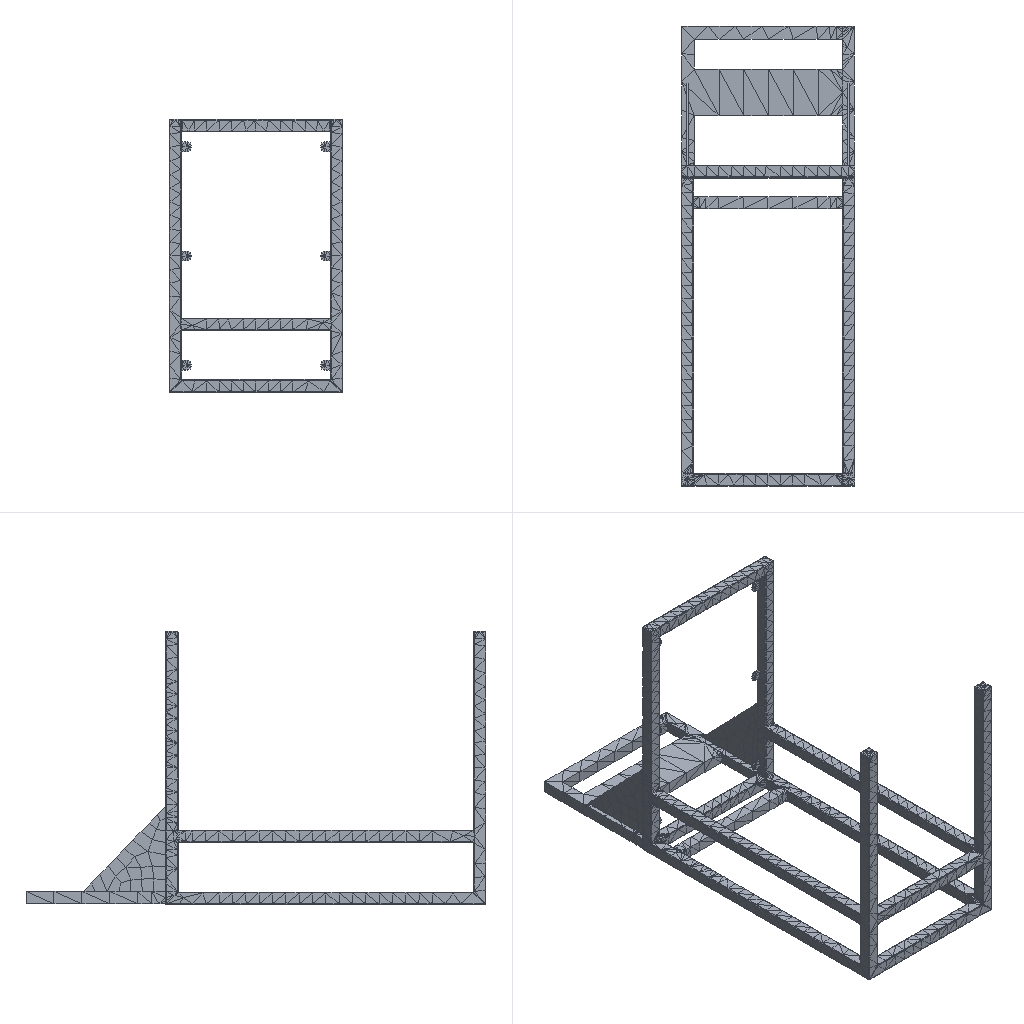Simulation study | ansys workbench
Ansys APDL input file, long lists of numbers shortened:
/batch
/config,noeldb,1     ! force off writing results to database
*get,_wallstrt,active,,time,wall
! ANSYS input file written by Workbench version 2022 R1
! File used for geometry attach: F:\ansys（分析文件汇总)\破碎机有限元分析\箱体.STEP
/title,wbnew--____ (D5)
! ****** Begin Custom Load Command Snippet ******
/COM, ACT Extensions:
/COM,     LSDYNA, 2021.1
/COM,
! ****** End   Custom Load Command Snippet ******
*DIM,_wb_ProjectScratch_dir,string,248
_wb_ProjectScratch_dir(1) = 'C:\Users\Administrator\AppData\Local\Temp\WB_Administrator_9184_2\_ProjectScratch\ScrCD4E\'
*DIM,_wb_SolverFiles_dir,string,248
_wb_SolverFiles_dir(1) = 'C:\Users\Administrator\AppData\Local\Temp\WB_Administrator_9184_2\wbnew_files\dp0\SYS-1\MECH\'
*DIM,_wb_userfiles_dir,string,248
_wb_userfiles_dir(1) = 'C:\Users\Administrator\AppData\Local\Temp\WB_Administrator_9184_2\wbnew_files\user_files\'
/com,--- Data in consistent NMM units. See Solving Units in the help system for more information.
/units,MPA
/nopr
/wb,file,start              !  signify a WB generated input file
/prep7
! Turn off shape checking because checks already performed inside WB mesher.
! See help system for more information.
SHPP,OFF,,NOWARN
/nolist
etcon,set             ! allow ANSYS to choose best KEYOP's for 180x elements, resets any applicable keyopt to MAPDL defaults
/com,*********** Nodes for the whole assembly ***********
nblock,3,,12097
(1i9,3e20.9e3)
        1    -1.386336680E+02     2.256626896E+02     1.867603707E+02
! (10997 more lines like these left out)
-1
/wb,elem,start            !  set before creation of elements
/com,*********** Elements for Body 1 "Part9_Assembly|LPattern1" ***********
et,1,186
keyo,1,2,1          ! set full integration on SOLID186
eblock,19,solid,,298
(19i9)
        1        1        1        1        0        0        0        0       20        0     1866     5561     5655     6044     5623     5854     5760     6063     5792
! (595 more lines like these left out)
-1
/com,*********** Elements for Body 2 "sideplates|Cut-Extrude5" ***********
et,2,187
eblock,19,solid,,1567
(19i9)
        2        2        2        2        0        0        0        0       10        0     2164     7986     8031     8115     8378     9370     9681     9371     9374
! (3133 more lines like these left out)
-1
/com,*********** Elements for Body 3 "sideplates|Cut-Extrude5[2]" ***********
et,3,187
eblock,19,solid,,1567
(19i9)
        3        3        3        3        0        0        0        0       10        0        1      139      184      268      531     1523     1834     1524     1527
! (3133 more lines like these left out)
-1
/com,*********** Elements for Body 4 "Part9_Assembly|LPattern1[2]" ***********
et,4,186
keyo,4,2,1          ! set full integration on SOLID186
eblock,19,solid,,298
(19i9)
        4        4        4        4        0        0        0        0       20        0     1568     3213     3307     3696     3275     3506     3412     3715     3444
! (595 more lines like these left out)
-1
/wb,elem,end               !  done creating elements
/com,*********** Send User Defined Coordinate System(s) ***********
csys,0
toffst,273.15,  ! Temperature offset from absolute zero
/com,*********** Set Reference Temperature ***********
tref,22.
/wb,mat,start              !  starting to send materials
/com,*********** Send Materials ***********
Temperature = 'TEMP' ! Temperature
MP,DENS,1,7.85e-09,	! tonne mm^-3
MP,ALPX,1,1.2e-05,	! C^-1
MP,C,1,434000000,	! mm^2 s^-2 C^-1
MP,KXX,1,60.5,	! tonne mm s^-3 C^-1
MP,RSVX,1,0.00017,	! ohm mm
MP,EX,1,200000,	! tonne s^-2 mm^-1
MP,NUXY,1,0.3,
MP,MURX,1,10000,
Temperature = 'TEMP' ! Temperature
MP,DENS,2,7.85e-09,	! tonne mm^-3
MP,ALPX,2,1.2e-05,	! C^-1
MP,C,2,434000000,	! mm^2 s^-2 C^-1
MP,KXX,2,60.5,	! tonne mm s^-3 C^-1
MP,RSVX,2,0.00017,	! ohm mm
MP,EX,2,200000,	! tonne s^-2 mm^-1
MP,NUXY,2,0.3,
MP,MURX,2,10000,
Temperature = 'TEMP' ! Temperature
MP,DENS,3,7.85e-09,	! tonne mm^-3
MP,ALPX,3,1.2e-05,	! C^-1
MP,C,3,434000000,	! mm^2 s^-2 C^-1
MP,KXX,3,60.5,	! tonne mm s^-3 C^-1
MP,RSVX,3,0.00017,	! ohm mm
MP,EX,3,200000,	! tonne s^-2 mm^-1
MP,NUXY,3,0.3,
MP,MURX,3,10000,
Temperature = 'TEMP' ! Temperature
MP,DENS,4,7.85e-09,	! tonne mm^-3
MP,ALPX,4,1.2e-05,	! C^-1
MP,C,4,434000000,	! mm^2 s^-2 C^-1
MP,KXX,4,60.5,	! tonne mm s^-3 C^-1
MP,RSVX,4,0.00017,	! ohm mm
MP,EX,4,200000,	! tonne s^-2 mm^-1
MP,NUXY,4,0.3,
MP,MURX,4,10000,
/wb,mat,end                !  done sending materials
!************************* Model Summary ********************
!Part9_Assembly|LPattern1,	结构钢,	matid,	1
!sideplates|Cut-Extrude5,	结构钢,	matid,	2
!sideplates|Cut-Extrude5[2],	结构钢,	matid,	3
!Part9_Assembly|LPattern1[2],	结构钢,	matid,	4
!************************* End Model Summary ********************
! get the diagonal of the bounding box. Needed later for other things
*get,_xmin,node,,mnloc,x
*get,_ymin,node,,mnloc,y
*get,_zmin,node,,mnloc,z
*get,_xmax,node,,mxloc,x
*get,_ymax,node,,mxloc,y
*get,_zmax,node,,mxloc,z
_ASMDIAG=(_xmax-_xmin)*(_xmax-_xmin)+(_ymax-_ymin)*(_ymax-_ymin)+(_zmax-_zmin)*(_zmax-_zmin)
_ASMDIAG=SQRT(_ASMDIAG)
/wb,contact,start          !  starting to send contact
/com,*********** Create Contact "接触区域" ***********
/com,            Real Constant Set For Above Contact Is 6 & 5
*set,tid,6
*set,cid,5
r,tid
r,cid
et,tid,170
et,cid,174
eblock,10,,,58
(15i9)
     7251        6        6        6        0     5930     5704     5650     5650     6900     6744     5650     6746
! (57 more lines like these left out)
-1
eblock,10,,,58
(15i9)
     7309        5        5        5        0     5930     5704     5650     5650     6900     6744     5650     6746
! (57 more lines like these left out)
-1
eblock,10,,,38
(15i9)
     7367        5        6        5        0     7850     7851     8116     8116     8393     8400     8116     8395
! (37 more lines like these left out)
-1
eblock,10,,,38
(15i9)
     7405        6        5        6        0     7850     7851     8116     8116     8393     8400     8116     8395
! (37 more lines like these left out)
-1
keyo,cid,8,2               ! auto create asymmetric contact (from Program Controlled setting)
keyo,cid,10,0              ! adjust contact stiffness each NR iteration (from Program Controlled setting)
keyo,cid,12,5              ! bonded always
keyo,cid,18,1              ! small sliding turned on by application
keyo,cid,2,0               ! augmented Lagrange (from Program Controlled setting)
keyo,cid,4,0               ! on Gauss point (from Program Controlled setting)
keyo,cid,9,1               ! ignore initial gaps/penetration
keyo,cid,7,0               ! No Prediction
rmod,tid,3,10.      ! FKN
rmod,tid,5,0.       ! ICONT
rmod,tid,6,0.       ! PINB
rmod,tid,10,0.      ! CNOF
rmod,tid,12,0.      ! FKT
rmod,tid,36,35      ! WB DSID
rmod,cid,3,10.      ! FKN
rmod,cid,5,0.       ! ICONT
rmod,cid,6,0.       ! PINB
rmod,cid,10,0.      ! CNOF
rmod,cid,12,0.      ! FKT
rmod,cid,36,35      ! WB DSID
/com,*********** Create Contact "接触区域 2" ***********
/com,            Real Constant Set For Above Contact Is 8 & 7
*set,tid,8
*set,cid,7
r,tid
r,cid
et,tid,170
et,cid,174
eblock,10,,,42
(15i9)
     7443        8        8        8        0     5657     5656     5658     5658     6768     6769     5658     6771
! (41 more lines like these left out)
-1
eblock,10,,,42
(15i9)
     7485        7        7        7        0     5657     5656     5658     5658     6768     6769     5658     6771
! (41 more lines like these left out)
-1
eblock,10,,,38
(15i9)
     7527        7        8        7        0        3        4      269      269      546      553      269      548
! (37 more lines like these left out)
-1
eblock,10,,,38
(15i9)
     7565        8        7        8        0        3        4      269      269      546      553      269      548
! (37 more lines like these left out)
-1
keyo,cid,8,2               ! auto create asymmetric contact (from Program Controlled setting)
keyo,cid,10,0              ! adjust contact stiffness each NR iteration (from Program Controlled setting)
keyo,cid,12,5              ! bonded always
keyo,cid,18,1              ! small sliding turned on by application
keyo,cid,2,0               ! augmented Lagrange (from Program Controlled setting)
keyo,cid,4,0               ! on Gauss point (from Program Controlled setting)
keyo,cid,9,1               ! ignore initial gaps/penetration
keyo,cid,7,0               ! No Prediction
rmod,tid,3,10.      ! FKN
rmod,tid,5,0.       ! ICONT
rmod,tid,6,0.       ! PINB
rmod,tid,10,0.      ! CNOF
rmod,tid,12,0.      ! FKT
rmod,tid,36,38      ! WB DSID
rmod,cid,3,10.      ! FKN
rmod,cid,5,0.       ! ICONT
rmod,cid,6,0.       ! PINB
rmod,cid,10,0.      ! CNOF
rmod,cid,12,0.      ! FKT
rmod,cid,36,38      ! WB DSID
/com,*********** Create Contact "接触区域 3" ***********
/com,            Real Constant Set For Above Contact Is 10 & 9
*set,tid,10
*set,cid,9
r,tid
r,cid
et,tid,170
et,cid,174
eblock,10,,,42
(15i9)
     7603       10       10       10        0     7908     8070     7909     7909     8852     8855     7909     8851
! (41 more lines like these left out)
-1
eblock,10,,,42
(15i9)
     7645        9        9        9        0     7908     8070     7909     7909     8852     8855     7909     8851
! (41 more lines like these left out)
-1
eblock,10,,,58
(15i9)
     7687        9       10        9        0     3829     3417     3363     3363     4770     4578     3363     4581
! (57 more lines like these left out)
-1
eblock,10,,,58
(15i9)
     7745       10        9       10        0     3829     3417     3363     3363     4770     4578     3363     4581
! (57 more lines like these left out)
-1
keyo,cid,8,2               ! auto create asymmetric contact (from Program Controlled setting)
keyo,cid,10,0              ! adjust contact stiffness each NR iteration (from Program Controlled setting)
keyo,cid,12,5              ! bonded always
keyo,cid,18,1              ! small sliding turned on by application
keyo,cid,2,0               ! augmented Lagrange (from Program Controlled setting)
keyo,cid,4,0               ! on Gauss point (from Program Controlled setting)
keyo,cid,9,1               ! ignore initial gaps/penetration
keyo,cid,7,0               ! No Prediction
rmod,tid,3,10.      ! FKN
rmod,tid,5,0.       ! ICONT
rmod,tid,6,0.       ! PINB
rmod,tid,10,0.      ! CNOF
rmod,tid,12,0.      ! FKT
rmod,tid,36,41      ! WB DSID
rmod,cid,3,10.      ! FKN
rmod,cid,5,0.       ! ICONT
rmod,cid,6,0.       ! PINB
rmod,cid,10,0.      ! CNOF
rmod,cid,12,0.      ! FKT
rmod,cid,36,41      ! WB DSID
/com,*********** Create Contact "接触区域 4" ***********
/com,            Real Constant Set For Above Contact Is 12 & 11
*set,tid,12
*set,cid,11
r,tid
r,cid
et,tid,170
et,cid,174
eblock,10,,,42
(15i9)
     7803       12       12       12        0       61      223       62       62     1005     1008       62     1004
! (41 more lines like these left out)
-1
eblock,10,,,42
(15i9)
     7845       11       11       11        0       61      223       62       62     1005     1008       62     1004
! (41 more lines like these left out)
-1
eblock,10,,,42
(15i9)
     7887       11       12       11        0     3410     3409     3411     3411     4741     4742     3411     4744
! (41 more lines like these left out)
-1
eblock,10,,,42
(15i9)
     7929       12       11       12        0     3410     3409     3411     3411     4741     4742     3411     4744
! (41 more lines like these left out)
-1
keyo,cid,8,2               ! auto create asymmetric contact (from Program Controlled setting)
keyo,cid,10,0              ! adjust contact stiffness each NR iteration (from Program Controlled setting)
keyo,cid,12,5              ! bonded always
keyo,cid,18,1              ! small sliding turned on by application
keyo,cid,2,0               ! augmented Lagrange (from Program Controlled setting)
keyo,cid,4,0               ! on Gauss point (from Program Controlled setting)
keyo,cid,9,1               ! ignore initial gaps/penetration
keyo,cid,7,0               ! No Prediction
rmod,tid,3,10.      ! FKN
rmod,tid,5,0.       ! ICONT
rmod,tid,6,0.       ! PINB
rmod,tid,10,0.      ! CNOF
rmod,tid,12,0.      ! FKT
rmod,tid,36,44      ! WB DSID
rmod,cid,3,10.      ! FKN
rmod,cid,5,0.       ! ICONT
rmod,cid,6,0.       ! PINB
rmod,cid,10,0.      ! CNOF
rmod,cid,12,0.      ! FKT
rmod,cid,36,44      ! WB DSID
nsel,all
esel,all
/wb,contact,end            !  done creating contacts
/golist
/wb,load,start             !  starting to send loads
/com,*********** Fixed Supports ***********
CMBLOCK,_FIXEDSU,NODE,      582
(8i10)
        81        82        83        84        85        86        87        88
! (72 more lines like these left out)
cmsel,s,_FIXEDSU
d,all,all
nsel,all
/com,*********** Define Force Using Surface Effect Elements ***********
local,12,0,0.,0.,0.,0.,0.,0.
csys,0
et,13,154
eblock,10,,,396
(15i9)
     7971       13       13       13       12      462      472      475      475     3061     3088      475     3062
! (395 more lines like these left out)
-1
esel,s,type,,13
keyop,13,2,1                ! Apply load in local coordinate system
keyop,13,7,1                ! Use original area so load is constant in large deformation
esel,all
/gst,on,on
fini
*get,_numnode,node,0,count
*get,_numelem,elem,0,count
*get, _MAXELEMNUM, elem, 0, NUM, MAX
*get, _MAXNODENUM, node, 0, NUM, MAX
*get, _MAXELEMTYPE, etyp, 0, NUM, MAX
*get, _MAXREALCONST, real, 0, NUM, MAX
/go
/wb,load,end               !  done creating loads
/com,--- Number of total nodes = %_numnode%
/com,--- Number of contact elements = 1116
/com,--- Number of spring elements = 0
/com,--- Number of bearing elements = 0
/com,--- Number of solid elements = 3730
/com,--- Number of condensed parts = 0
/com,--- Number of total elements = %_numelem%
*get,_wallbsol,active,,time,wall
/com,****************************************************************************
/com,*************************    SOLUTION       ********************************
/com,****************************************************************************
/solu
antype,0                   ! static analysis
_thickRatio=  0     ! Ratio of thick parts in the model
eqsl,sparse,,,,,1
cntr,print,1               ! print out contact info and also make no initial contact an error
dmpoption,emat,no             ! Don't combine emat file for DANSYS
dmpoption,esav,no             ! Don't combine esav file for DANSYS
nldiag,cont,iter           ! print out contact info each equilibrium iteration
rescontrol,,none                 ! Do not keep any restart files
/com,****************************************************
/com,******************* SOLVE FOR LS 1 OF 1 ****************
esel,s,type,,13
nsle
sfe,all,1,pres,1,0.
sfe,all,2,pres,1,-0.1946
sfe,all,3,pres,1,0.
nsel,all
esel,all
/nopr
/gopr
nsub,1,1,1
time,1.
outres,erase
outres,all,none
outres,nsol,all,
outres,rsol,all
outres,eangl,all
outres,etmp,all
outres,veng,all
outres,strs,all,
outres,epel,all,
outres,eppl,all,
outres,cont,all,
! *********** WB SOLVE COMMAND ***********
! check interactive state
*get,ANSINTER_,active,,int
*if,ANSINTER_,ne,0,then
/eof
*endif
solve
/com *************** Write FE CONNECTORS *********
CEWRITE,file,ce,,INTE
/com,****************************************************
/com,*************** FINISHED SOLVE FOR LS 1 *************
*get,_wallasol,active,,time,wall
/nopr
*get,_numnode,node,0,count
*get,_numelem,elem,0,count
*get, _MAXELEMNUM, elem, 0, NUM, MAX
*get, _MAXNODENUM, node, 0, NUM, MAX,,,INTERNAL
*get, _MAXELEMTYPE, etyp, 0, NUM, MAX
*get, _MAXREALCONST, real, 0, NUM, MAX
/gopr
/post1
xmlo,ENCODING,ISO-8859-1
xmlo,parm
/xml,parm,xml
fini
/gopr
*get,_walldone,active,,time,wall
_preptime=(_wallbsol-_wallstrt)*3600
_solvtime=(_wallasol-_wallbsol)*3600
_posttime=(_walldone-_wallasol)*3600
_totaltim=(_walldone-_wallstrt)*3600
*get,_dlbratio,active,0,solu,dlbr
*get,_combtime,active,0,solu,comb
*get,_ssmode,active,0,solu,ssmm
*get,_ndofs,active,0,solu,ndof
*get,_sol_end_time,active,0,set,time
*if,_sol_end_time,eq,1.,then
/fclean				!clean distributed files
*endif
/com,--- Total number of nodes = %_numnode%
/com,--- Total number of elements = %_numelem%
/com,--- Element load balance ratio = %_dlbratio%
/com,--- Time to combine distributed files = %_combtime%
/com,--- Sparse memory mode = %_ssmode%
/com,--- Number of DOF = %_ndofs%
/wb,file,end               ! done with WB generated input